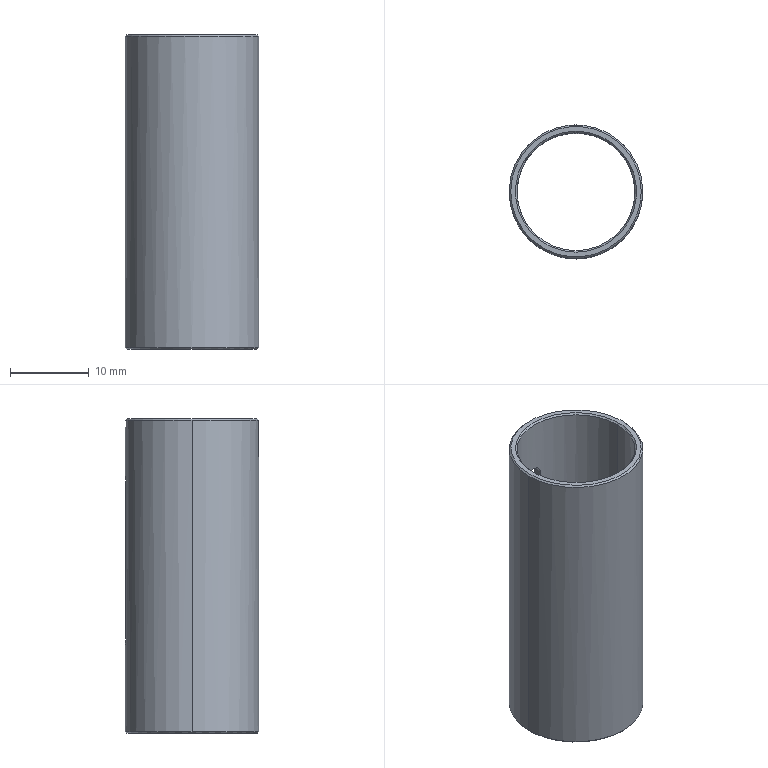Part | SolidWorks | features BaseBody 1, MoveFace 1 | 1 solid | 25 faces | box 17 x 17 x 40 mm | volume 1956 mm3 | cone 12 | cylinder 9 | plane 4 | commonest cylinder face diameters 15 x4 2 x3 17 x2
STEP:
#1=CARTESIAN_POINT('',(-1.,8.441,12.));
#2=VERTEX_POINT('',#1);
#3=CARTESIAN_POINT('',(0.,8.5,11.));
#4=VERTEX_POINT('',#3);
#5=CARTESIAN_POINT('',(-1.,8.441,12.));
#6=CARTESIAN_POINT('',(-1.,8.441,11.868));
#7=CARTESIAN_POINT('',(-0.9739,8.444,11.738));
#8=CARTESIAN_POINT('',(-0.8734,8.455,11.496));
#9=CARTESIAN_POINT('',(-0.7991,8.463,11.385));
#10=CARTESIAN_POINT('',(-0.6146,8.478,11.2));
#11=CARTESIAN_POINT('',(-0.5031,8.486,11.126));
#12=CARTESIAN_POINT('',(-0.2623,8.497,11.026));
#13=CARTESIAN_POINT('',(-0.1306,8.5,11.));
#14=CARTESIAN_POINT('',(0.,8.5,11.));
#15=B_SPLINE_CURVE_WITH_KNOTS('',3,(#5,#6,#7,#8,#9,#10,#11,#12,#13,#14),.UNSPECIFIED.,.F.,.F.,(4,2,2,2,4),(0.,0.0003912,0.0007825,0.001174,0.001565),.UNSPECIFIED.);
#16=EDGE_CURVE('',#2,#4,#15,.T.);
#17=ORIENTED_EDGE('',*,*,#16,.T.);
#18=CARTESIAN_POINT('',(1.,8.441,12.));
#19=VERTEX_POINT('',#18);
#20=CARTESIAN_POINT('',(0.,8.5,11.));
#21=CARTESIAN_POINT('',(0.1305,8.5,11.));
#22=CARTESIAN_POINT('',(0.2615,8.497,11.026));
#23=CARTESIAN_POINT('',(0.5036,8.486,11.126));
#24=CARTESIAN_POINT('',(0.6136,8.478,11.199));
#25=CARTESIAN_POINT('',(0.8002,8.463,11.386));
#26=CARTESIAN_POINT('',(0.8735,8.455,11.496));
#27=CARTESIAN_POINT('',(0.9739,8.444,11.738));
#28=CARTESIAN_POINT('',(1.,8.441,11.868));
#29=CARTESIAN_POINT('',(1.,8.441,12.));
#30=B_SPLINE_CURVE_WITH_KNOTS('',3,(#20,#21,#22,#23,#24,#25,#26,#27,#28,#29),.UNSPECIFIED.,.F.,.F.,(4,2,2,2,4),(0.001565,0.001956,0.002347,0.002738,0.003128),.UNSPECIFIED.);
#31=EDGE_CURVE('',#4,#19,#30,.T.);
#32=ORIENTED_EDGE('',*,*,#31,.T.);
#33=CARTESIAN_POINT('',(1.,8.441,32.));
#34=VERTEX_POINT('',#33);
#35=CARTESIAN_POINT('',(1.,8.441,40.));
#36=DIRECTION('',(0.,0.,1.));
#37=VECTOR('',#36,1000.);
#38=LINE('',#35,#37);
#39=EDGE_CURVE('',#19,#34,#38,.T.);
#40=ORIENTED_EDGE('',*,*,#39,.T.);
#41=CARTESIAN_POINT('',(-1.,8.441,32.));
#42=VERTEX_POINT('',#41);
#43=CARTESIAN_POINT('',(1.,8.441,32.));
#44=CARTESIAN_POINT('',(1.,8.441,32.132));
#45=CARTESIAN_POINT('',(0.9739,8.444,32.262));
#46=CARTESIAN_POINT('',(0.8735,8.455,32.504));
#47=CARTESIAN_POINT('',(0.7992,8.463,32.615));
#48=CARTESIAN_POINT('',(0.6149,8.478,32.799));
#49=CARTESIAN_POINT('',(0.5035,8.486,32.874));
#50=CARTESIAN_POINT('',(0.2629,8.497,32.974));
#51=CARTESIAN_POINT('',(0.1313,8.5,33.));
#52=CARTESIAN_POINT('',(-0.1298,8.5,33.));
#53=CARTESIAN_POINT('',(-0.2609,8.497,32.974));
#54=CARTESIAN_POINT('',(-0.5032,8.486,32.874));
#55=CARTESIAN_POINT('',(-0.6133,8.478,32.801));
#56=CARTESIAN_POINT('',(-0.8,8.463,32.614));
#57=CARTESIAN_POINT('',(-0.8734,8.455,32.504));
#58=CARTESIAN_POINT('',(-0.9738,8.444,32.262));
#59=CARTESIAN_POINT('',(-1.,8.441,32.132));
#60=CARTESIAN_POINT('',(-1.,8.441,32.));
#61=B_SPLINE_CURVE_WITH_KNOTS('',3,(#43,#44,#45,#46,#47,#48,#49,#50,#51,#52,#53,#54,#55,#56,#57,#58,#59,#60),.UNSPECIFIED.,.F.,.F.,(4,2,2,2,2,2,2,2,4),(0.,0.0003911,0.0007821,0.001173,0.001564,0.001955,0.002346,0.002737,0.003128),.UNSPECIFIED.);
#62=EDGE_CURVE('',#34,#42,#61,.T.);
#63=ORIENTED_EDGE('',*,*,#62,.T.);
#64=CARTESIAN_POINT('',(-1.,8.441,40.));
#65=DIRECTION('',(0.,0.,-1.));
#66=VECTOR('',#65,1000.);
#67=LINE('',#64,#66);
#68=EDGE_CURVE('',#42,#2,#67,.T.);
#69=ORIENTED_EDGE('',*,*,#68,.T.);
#70=EDGE_LOOP('',(#17,#32,#40,#63,#69));
#71=FACE_BOUND('',#70,.T.);
#72=CARTESIAN_POINT('',(-8.5,0.,39.8));
#73=VERTEX_POINT('',#72);
#74=CARTESIAN_POINT('',(8.5,0.,39.8));
#75=VERTEX_POINT('',#74);
#76=CARTESIAN_POINT('',(0.,0.,39.8));
#77=DIRECTION('',(0.,0.,-1.));
#78=DIRECTION('',(-1.,0.,0.));
#79=AXIS2_PLACEMENT_3D('',#76,#77,#78);
#80=CIRCLE('',#79,8.5);
#81=EDGE_CURVE('',#73,#75,#80,.T.);
#82=ORIENTED_EDGE('',*,*,#81,.T.);
#83=CARTESIAN_POINT('',(8.5,0.,0.2));
#84=VERTEX_POINT('',#83);
#85=CARTESIAN_POINT('',(8.5,0.,40.));
#86=DIRECTION('',(0.,0.,-1.));
#87=VECTOR('',#86,1000.);
#88=LINE('',#85,#87);
#89=EDGE_CURVE('',#75,#84,#88,.T.);
#90=ORIENTED_EDGE('',*,*,#89,.T.);
#91=CARTESIAN_POINT('',(0.,8.5,0.2));
#92=VERTEX_POINT('',#91);
#93=CARTESIAN_POINT('',(0.,0.,0.2));
#94=DIRECTION('',(0.,0.,1.));
#95=DIRECTION('',(-1.,0.,0.));
#96=AXIS2_PLACEMENT_3D('',#93,#94,#95);
#97=CIRCLE('',#96,8.5);
#98=EDGE_CURVE('',#84,#92,#97,.T.);
#99=ORIENTED_EDGE('',*,*,#98,.T.);
#100=CARTESIAN_POINT('',(-8.5,0.,0.2));
#101=VERTEX_POINT('',#100);
#102=CARTESIAN_POINT('',(0.,0.,0.2));
#103=DIRECTION('',(0.,0.,1.));
#104=DIRECTION('',(-1.,0.,0.));
#105=AXIS2_PLACEMENT_3D('',#102,#103,#104);
#106=CIRCLE('',#105,8.5);
#107=EDGE_CURVE('',#92,#101,#106,.T.);
#108=ORIENTED_EDGE('',*,*,#107,.T.);
#109=CARTESIAN_POINT('',(-8.5,0.,40.));
#110=DIRECTION('',(0.,0.,-1.));
#111=VECTOR('',#110,1000.);
#112=LINE('',#109,#111);
#113=EDGE_CURVE('',#73,#101,#112,.T.);
#114=ORIENTED_EDGE('',*,*,#113,.F.);
#115=EDGE_LOOP('',(#82,#90,#99,#108,#114));
#116=FACE_OUTER_BOUND('',#115,.T.);
#117=CARTESIAN_POINT('',(0.,0.,40.));
#118=DIRECTION('',(0.,0.,-1.));
#119=DIRECTION('',(-1.,0.,0.));
#120=AXIS2_PLACEMENT_3D('',#117,#118,#119);
#121=CYLINDRICAL_SURFACE('',#120,8.5);
#122=ADVANCED_FACE('',(#71,#116),#121,.T.);
#123=CARTESIAN_POINT('',(0.,-8.3,0.));
#124=VERTEX_POINT('',#123);
#125=CARTESIAN_POINT('',(0.,8.3,0.));
#126=VERTEX_POINT('',#125);
#127=CARTESIAN_POINT('',(0.,0.,0.));
#128=DIRECTION('',(0.,0.,1.));
#129=DIRECTION('',(0.,-1.,0.));
#130=AXIS2_PLACEMENT_3D('',#127,#128,#129);
#131=CIRCLE('',#130,8.3);
#132=EDGE_CURVE('',#124,#126,#131,.T.);
#133=ORIENTED_EDGE('',*,*,#132,.T.);
#134=CARTESIAN_POINT('',(0.,8.5,0.2));
#135=DIRECTION('',(0.,0.7071,0.7071));
#136=VECTOR('',#135,1000.);
#137=LINE('',#134,#136);
#138=EDGE_CURVE('',#126,#92,#137,.T.);
#139=ORIENTED_EDGE('',*,*,#138,.T.);
#140=ORIENTED_EDGE('',*,*,#98,.F.);
#141=CARTESIAN_POINT('',(0.,-8.5,0.2));
#142=VERTEX_POINT('',#141);
#143=CARTESIAN_POINT('',(0.,0.,0.2));
#144=DIRECTION('',(0.,0.,1.));
#145=DIRECTION('',(-1.,0.,0.));
#146=AXIS2_PLACEMENT_3D('',#143,#144,#145);
#147=CIRCLE('',#146,8.5);
#148=EDGE_CURVE('',#142,#84,#147,.T.);
#149=ORIENTED_EDGE('',*,*,#148,.F.);
#150=CARTESIAN_POINT('',(0.,-8.5,0.2));
#151=DIRECTION('',(0.,-0.7071,0.7071));
#152=VECTOR('',#151,1000.);
#153=LINE('',#150,#152);
#154=EDGE_CURVE('',#124,#142,#153,.T.);
#155=ORIENTED_EDGE('',*,*,#154,.F.);
#156=EDGE_LOOP('',(#133,#139,#140,#149,#155));
#157=FACE_OUTER_BOUND('',#156,.T.);
#158=CARTESIAN_POINT('',(0.,0.,0.2));
#159=DIRECTION('',(0.,0.,1.));
#160=DIRECTION('',(0.,-1.,0.));
#161=AXIS2_PLACEMENT_3D('',#158,#159,#160);
#162=CONICAL_SURFACE('',#161,8.5,0.7854);
#163=ADVANCED_FACE('',(#157),#162,.T.);
#164=CARTESIAN_POINT('',(-8.3,0.,40.));
#165=VERTEX_POINT('',#164);
#166=CARTESIAN_POINT('',(8.3,0.,40.));
#167=VERTEX_POINT('',#166);
#168=CARTESIAN_POINT('',(0.,0.,40.));
#169=DIRECTION('',(0.,0.,-1.));
#170=DIRECTION('',(-1.,0.,0.));
#171=AXIS2_PLACEMENT_3D('',#168,#169,#170);
#172=CIRCLE('',#171,8.3);
#173=EDGE_CURVE('',#165,#167,#172,.T.);
#174=ORIENTED_EDGE('',*,*,#173,.T.);
#175=CARTESIAN_POINT('',(8.5,0.,39.8));
#176=DIRECTION('',(0.7071,0.,-0.7071));
#177=VECTOR('',#176,1000.);
#178=LINE('',#175,#177);
#179=EDGE_CURVE('',#167,#75,#178,.T.);
#180=ORIENTED_EDGE('',*,*,#179,.T.);
#181=ORIENTED_EDGE('',*,*,#81,.F.);
#182=CARTESIAN_POINT('',(-8.5,0.,39.8));
#183=DIRECTION('',(-0.7071,0.,-0.7071));
#184=VECTOR('',#183,1000.);
#185=LINE('',#182,#184);
#186=EDGE_CURVE('',#165,#73,#185,.T.);
#187=ORIENTED_EDGE('',*,*,#186,.F.);
#188=EDGE_LOOP('',(#174,#180,#181,#187));
#189=FACE_OUTER_BOUND('',#188,.T.);
#190=CARTESIAN_POINT('',(0.,0.,39.8));
#191=DIRECTION('',(0.,0.,-1.));
#192=DIRECTION('',(-1.,0.,0.));
#193=AXIS2_PLACEMENT_3D('',#190,#191,#192);
#194=CONICAL_SURFACE('',#193,8.5,0.7854);
#195=ADVANCED_FACE('',(#189),#194,.T.);
#196=ORIENTED_EDGE('',*,*,#31,.F.);
#197=CARTESIAN_POINT('',(0.,7.5,11.));
#198=VERTEX_POINT('',#197);
#199=CARTESIAN_POINT('',(0.,8.5,11.));
#200=DIRECTION('',(0.,-1.,0.));
#201=VECTOR('',#200,1000.);
#202=LINE('',#199,#201);
#203=EDGE_CURVE('',#4,#198,#202,.T.);
#204=ORIENTED_EDGE('',*,*,#203,.T.);
#205=CARTESIAN_POINT('',(1.,7.433,12.));
#206=VERTEX_POINT('',#205);
#207=CARTESIAN_POINT('',(1.,7.433,12.));
#208=CARTESIAN_POINT('',(1.,7.433,11.868));
#209=CARTESIAN_POINT('',(0.9739,7.437,11.738));
#210=CARTESIAN_POINT('',(0.8734,7.449,11.496));
#211=CARTESIAN_POINT('',(0.799,7.458,11.385));
#212=CARTESIAN_POINT('',(0.6146,7.475,11.2));
#213=CARTESIAN_POINT('',(0.5031,7.484,11.126));
#214=CARTESIAN_POINT('',(0.2624,7.496,11.026));
#215=CARTESIAN_POINT('',(0.1306,7.5,11.));
#216=CARTESIAN_POINT('',(0.,7.5,11.));
#217=B_SPLINE_CURVE_WITH_KNOTS('',3,(#207,#208,#209,#210,#211,#212,#213,#214,#215,#216),.UNSPECIFIED.,.F.,.F.,(4,2,2,2,4),(0.,0.0003913,0.0007827,0.001174,0.001565),.UNSPECIFIED.);
#218=EDGE_CURVE('',#206,#198,#217,.T.);
#219=ORIENTED_EDGE('',*,*,#218,.F.);
#220=CARTESIAN_POINT('',(1.,8.5,12.));
#221=DIRECTION('',(0.,-1.,0.));
#222=VECTOR('',#221,1000.);
#223=LINE('',#220,#222);
#224=EDGE_CURVE('',#19,#206,#223,.T.);
#225=ORIENTED_EDGE('',*,*,#224,.F.);
#226=EDGE_LOOP('',(#196,#204,#219,#225));
#227=FACE_OUTER_BOUND('',#226,.T.);
#228=CARTESIAN_POINT('',(0.,8.5,12.));
#229=DIRECTION('',(0.,-1.,0.));
#230=DIRECTION('',(0.,0.,-1.));
#231=AXIS2_PLACEMENT_3D('',#228,#229,#230);
#232=CYLINDRICAL_SURFACE('',#231,1.);
#233=ADVANCED_FACE('',(#227),#232,.F.);
#234=CARTESIAN_POINT('',(7.5,0.,0.2));
#235=VERTEX_POINT('',#234);
#236=CARTESIAN_POINT('',(-7.5,0.,0.2));
#237=VERTEX_POINT('',#236);
#238=CARTESIAN_POINT('',(0.,0.,0.2));
#239=DIRECTION('',(0.,0.,-1.));
#240=DIRECTION('',(-1.,0.,0.));
#241=AXIS2_PLACEMENT_3D('',#238,#239,#240);
#242=CIRCLE('',#241,7.5);
#243=EDGE_CURVE('',#235,#237,#242,.T.);
#244=ORIENTED_EDGE('',*,*,#243,.F.);
#245=CARTESIAN_POINT('',(7.7,0.,0.));
#246=VERTEX_POINT('',#245);
#247=CARTESIAN_POINT('',(7.7,0.,0.));
#248=DIRECTION('',(0.7071,0.,-0.7071));
#249=VECTOR('',#248,1000.);
#250=LINE('',#247,#249);
#251=EDGE_CURVE('',#235,#246,#250,.T.);
#252=ORIENTED_EDGE('',*,*,#251,.T.);
#253=CARTESIAN_POINT('',(-7.7,0.,0.));
#254=VERTEX_POINT('',#253);
#255=CARTESIAN_POINT('',(0.,0.,0.));
#256=DIRECTION('',(0.,0.,-1.));
#257=DIRECTION('',(-1.,0.,0.));
#258=AXIS2_PLACEMENT_3D('',#255,#256,#257);
#259=CIRCLE('',#258,7.7);
#260=EDGE_CURVE('',#246,#254,#259,.T.);
#261=ORIENTED_EDGE('',*,*,#260,.T.);
#262=CARTESIAN_POINT('',(-7.7,0.,0.));
#263=DIRECTION('',(-0.7071,0.,-0.7071));
#264=VECTOR('',#263,1000.);
#265=LINE('',#262,#264);
#266=EDGE_CURVE('',#237,#254,#265,.T.);
#267=ORIENTED_EDGE('',*,*,#266,.F.);
#268=EDGE_LOOP('',(#244,#252,#261,#267));
#269=FACE_OUTER_BOUND('',#268,.T.);
#270=CARTESIAN_POINT('',(0.,0.,0.));
#271=DIRECTION('',(0.,0.,-1.));
#272=DIRECTION('',(-1.,0.,0.));
#273=AXIS2_PLACEMENT_3D('',#270,#271,#272);
#274=CONICAL_SURFACE('',#273,7.7,0.7854);
#275=ADVANCED_FACE('',(#269),#274,.F.);
#276=CARTESIAN_POINT('',(7.5,0.,39.8));
#277=VERTEX_POINT('',#276);
#278=CARTESIAN_POINT('',(0.,-7.5,39.8));
#279=VERTEX_POINT('',#278);
#280=CARTESIAN_POINT('',(0.,0.,39.8));
#281=DIRECTION('',(0.,0.,-1.));
#282=DIRECTION('',(-1.,0.,0.));
#283=AXIS2_PLACEMENT_3D('',#280,#281,#282);
#284=CIRCLE('',#283,7.5);
#285=EDGE_CURVE('',#277,#279,#284,.T.);
#286=ORIENTED_EDGE('',*,*,#285,.F.);
#287=CARTESIAN_POINT('',(7.5,0.,2.289));
#288=VERTEX_POINT('',#287);
#289=CARTESIAN_POINT('',(7.5,0.,40.));
#290=DIRECTION('',(0.,0.,-1.));
#291=VECTOR('',#290,1000.);
#292=LINE('',#289,#291);
#293=EDGE_CURVE('',#277,#288,#292,.T.);
#294=ORIENTED_EDGE('',*,*,#293,.T.);
#295=CARTESIAN_POINT('',(-7.5,0.,2.289));
#296=VERTEX_POINT('',#295);
#297=CARTESIAN_POINT('',(0.,0.,2.289));
#298=DIRECTION('',(0.,0.,1.));
#299=DIRECTION('',(-1.,0.,0.));
#300=AXIS2_PLACEMENT_3D('',#297,#298,#299);
#301=CIRCLE('',#300,7.5);
#302=EDGE_CURVE('',#296,#288,#301,.T.);
#303=ORIENTED_EDGE('',*,*,#302,.F.);
#304=CARTESIAN_POINT('',(-7.5,0.,39.8));
#305=VERTEX_POINT('',#304);
#306=CARTESIAN_POINT('',(-7.5,0.,40.));
#307=DIRECTION('',(0.,0.,-1.));
#308=VECTOR('',#307,1000.);
#309=LINE('',#306,#308);
#310=EDGE_CURVE('',#305,#296,#309,.T.);
#311=ORIENTED_EDGE('',*,*,#310,.F.);
#312=CARTESIAN_POINT('',(0.,0.,39.8));
#313=DIRECTION('',(0.,0.,-1.));
#314=DIRECTION('',(-1.,0.,0.));
#315=AXIS2_PLACEMENT_3D('',#312,#313,#314);
#316=CIRCLE('',#315,7.5);
#317=EDGE_CURVE('',#279,#305,#316,.T.);
#318=ORIENTED_EDGE('',*,*,#317,.F.);
#319=EDGE_LOOP('',(#286,#294,#303,#311,#318));
#320=FACE_OUTER_BOUND('',#319,.T.);
#321=CARTESIAN_POINT('',(0.,0.,40.));
#322=DIRECTION('',(0.,0.,-1.));
#323=DIRECTION('',(-1.,0.,0.));
#324=AXIS2_PLACEMENT_3D('',#321,#322,#323);
#325=CYLINDRICAL_SURFACE('',#324,7.5);
#326=ADVANCED_FACE('',(#320),#325,.F.);
#327=ORIENTED_EDGE('',*,*,#317,.T.);
#328=CARTESIAN_POINT('',(0.,7.5,39.8));
#329=VERTEX_POINT('',#328);
#330=CARTESIAN_POINT('',(0.,0.,39.8));
#331=DIRECTION('',(0.,0.,-1.));
#332=DIRECTION('',(-1.,0.,0.));
#333=AXIS2_PLACEMENT_3D('',#330,#331,#332);
#334=CIRCLE('',#333,7.5);
#335=EDGE_CURVE('',#305,#329,#334,.T.);
#336=ORIENTED_EDGE('',*,*,#335,.T.);
#337=CARTESIAN_POINT('',(0.,7.7,40.));
#338=VERTEX_POINT('',#337);
#339=CARTESIAN_POINT('',(0.,7.7,40.));
#340=DIRECTION('',(0.,0.7071,0.7071));
#341=VECTOR('',#340,1000.);
#342=LINE('',#339,#341);
#343=EDGE_CURVE('',#329,#338,#342,.T.);
#344=ORIENTED_EDGE('',*,*,#343,.T.);
#345=CARTESIAN_POINT('',(0.,-7.7,40.));
#346=VERTEX_POINT('',#345);
#347=CARTESIAN_POINT('',(0.,0.,40.));
#348=DIRECTION('',(0.,0.,-1.));
#349=DIRECTION('',(0.,-1.,0.));
#350=AXIS2_PLACEMENT_3D('',#347,#348,#349);
#351=CIRCLE('',#350,7.7);
#352=EDGE_CURVE('',#346,#338,#351,.T.);
#353=ORIENTED_EDGE('',*,*,#352,.F.);
#354=CARTESIAN_POINT('',(0.,-7.7,40.));
#355=DIRECTION('',(0.,-0.7071,0.7071));
#356=VECTOR('',#355,1000.);
#357=LINE('',#354,#356);
#358=EDGE_CURVE('',#279,#346,#357,.T.);
#359=ORIENTED_EDGE('',*,*,#358,.F.);
#360=EDGE_LOOP('',(#327,#336,#344,#353,#359));
#361=FACE_OUTER_BOUND('',#360,.T.);
#362=CARTESIAN_POINT('',(0.,0.,40.));
#363=DIRECTION('',(0.,0.,1.));
#364=DIRECTION('',(0.,-1.,0.));
#365=AXIS2_PLACEMENT_3D('',#362,#363,#364);
#366=CONICAL_SURFACE('',#365,7.7,0.7854);
#367=ADVANCED_FACE('',(#361),#366,.F.);
#368=CARTESIAN_POINT('',(7.5,0.,1.711));
#369=VERTEX_POINT('',#368);
#370=CARTESIAN_POINT('',(-7.5,0.,1.711));
#371=VERTEX_POINT('',#370);
#372=CARTESIAN_POINT('',(0.,0.,1.711));
#373=DIRECTION('',(0.,0.,-1.));
#374=DIRECTION('',(-1.,0.,0.));
#375=AXIS2_PLACEMENT_3D('',#372,#373,#374);
#376=CIRCLE('',#375,7.5);
#377=EDGE_CURVE('',#369,#371,#376,.T.);
#378=ORIENTED_EDGE('',*,*,#377,.F.);
#379=CARTESIAN_POINT('',(7.5,0.,40.));
#380=DIRECTION('',(0.,0.,-1.));
#381=VECTOR('',#380,1000.);
#382=LINE('',#379,#381);
#383=EDGE_CURVE('',#369,#235,#382,.T.);
#384=ORIENTED_EDGE('',*,*,#383,.T.);
#385=ORIENTED_EDGE('',*,*,#243,.T.);
#386=CARTESIAN_POINT('',(-7.5,0.,40.));
#387=DIRECTION('',(0.,0.,-1.));
#388=VECTOR('',#387,1000.);
#389=LINE('',#386,#388);
#390=EDGE_CURVE('',#371,#237,#389,.T.);
#391=ORIENTED_EDGE('',*,*,#390,.F.);
#392=EDGE_LOOP('',(#378,#384,#385,#391));
#393=FACE_OUTER_BOUND('',#392,.T.);
#394=CARTESIAN_POINT('',(0.,0.,40.));
#395=DIRECTION('',(0.,0.,-1.));
#396=DIRECTION('',(-1.,0.,0.));
#397=AXIS2_PLACEMENT_3D('',#394,#395,#396);
#398=CYLINDRICAL_SURFACE('',#397,7.5);
#399=ADVANCED_FACE('',(#393),#398,.F.);
#400=ORIENTED_EDGE('',*,*,#302,.T.);
#401=CARTESIAN_POINT('',(8.,0.,2.));
#402=VERTEX_POINT('',#401);
#403=CARTESIAN_POINT('',(8.,0.,2.));
#404=DIRECTION('',(0.866,0.,-0.5));
#405=VECTOR('',#404,1000.);
#406=LINE('',#403,#405);
#407=EDGE_CURVE('',#288,#402,#406,.T.);
#408=ORIENTED_EDGE('',*,*,#407,.T.);
#409=CARTESIAN_POINT('',(-8.,0.,2.));
#410=VERTEX_POINT('',#409);
#411=CARTESIAN_POINT('',(0.,0.,2.));
#412=DIRECTION('',(0.,0.,1.));
#413=DIRECTION('',(-1.,0.,0.));
#414=AXIS2_PLACEMENT_3D('',#411,#412,#413);
#415=CIRCLE('',#414,8.);
#416=EDGE_CURVE('',#410,#402,#415,.T.);
#417=ORIENTED_EDGE('',*,*,#416,.F.);
#418=CARTESIAN_POINT('',(-8.,0.,2.));
#419=DIRECTION('',(-0.866,0.,-0.5));
#420=VECTOR('',#419,1000.);
#421=LINE('',#418,#420);
#422=EDGE_CURVE('',#296,#410,#421,.T.);
#423=ORIENTED_EDGE('',*,*,#422,.F.);
#424=EDGE_LOOP('',(#400,#408,#417,#423));
#425=FACE_OUTER_BOUND('',#424,.T.);
#426=CARTESIAN_POINT('',(0.,0.,2.));
#427=DIRECTION('',(0.,0.,-1.));
#428=DIRECTION('',(-1.,0.,0.));
#429=AXIS2_PLACEMENT_3D('',#426,#427,#428);
#430=CONICAL_SURFACE('',#429,8.,1.047);
#431=ADVANCED_FACE('',(#425),#430,.F.);
#432=ORIENTED_EDGE('',*,*,#377,.T.);
#433=CARTESIAN_POINT('',(-8.,0.,2.));
#434=DIRECTION('',(-0.866,0.,0.5));
#435=VECTOR('',#434,1000.);
#436=LINE('',#433,#435);
#437=EDGE_CURVE('',#371,#410,#436,.T.);
#438=ORIENTED_EDGE('',*,*,#437,.T.);
#439=ORIENTED_EDGE('',*,*,#416,.T.);
#440=CARTESIAN_POINT('',(8.,0.,2.));
#441=DIRECTION('',(0.866,0.,0.5));
#442=VECTOR('',#441,1000.);
#443=LINE('',#440,#442);
#444=EDGE_CURVE('',#369,#402,#443,.T.);
#445=ORIENTED_EDGE('',*,*,#444,.F.);
#446=EDGE_LOOP('',(#432,#438,#439,#445));
#447=FACE_OUTER_BOUND('',#446,.T.);
#448=CARTESIAN_POINT('',(0.,0.,2.));
#449=DIRECTION('',(0.,0.,1.));
#450=DIRECTION('',(1.,0.,0.));
#451=AXIS2_PLACEMENT_3D('',#448,#449,#450);
#452=CONICAL_SURFACE('',#451,8.,1.047);
#453=ADVANCED_FACE('',(#447),#452,.F.);
#454=ORIENTED_EDGE('',*,*,#89,.F.);
#455=CARTESIAN_POINT('',(0.,0.,39.8));
#456=DIRECTION('',(0.,0.,-1.));
#457=DIRECTION('',(-1.,0.,0.));
#458=AXIS2_PLACEMENT_3D('',#455,#456,#457);
#459=CIRCLE('',#458,8.5);
#460=EDGE_CURVE('',#75,#73,#459,.T.);
#461=ORIENTED_EDGE('',*,*,#460,.T.);
#462=ORIENTED_EDGE('',*,*,#113,.T.);
#463=CARTESIAN_POINT('',(0.,0.,0.2));
#464=DIRECTION('',(0.,0.,1.));
#465=DIRECTION('',(-1.,0.,0.));
#466=AXIS2_PLACEMENT_3D('',#463,#464,#465);
#467=CIRCLE('',#466,8.5);
#468=EDGE_CURVE('',#101,#142,#467,.T.);
#469=ORIENTED_EDGE('',*,*,#468,.T.);
#470=ORIENTED_EDGE('',*,*,#148,.T.);
#471=EDGE_LOOP('',(#454,#461,#462,#469,#470));
#472=FACE_OUTER_BOUND('',#471,.T.);
#473=CARTESIAN_POINT('',(0.,0.,40.));
#474=DIRECTION('',(0.,0.,-1.));
#475=DIRECTION('',(-1.,0.,0.));
#476=AXIS2_PLACEMENT_3D('',#473,#474,#475);
#477=CYLINDRICAL_SURFACE('',#476,8.5);
#478=ADVANCED_FACE('',(#472),#477,.T.);
#479=ORIENTED_EDGE('',*,*,#138,.F.);
#480=CARTESIAN_POINT('',(0.,0.,0.));
#481=DIRECTION('',(0.,0.,1.));
#482=DIRECTION('',(0.,-1.,0.));
#483=AXIS2_PLACEMENT_3D('',#480,#481,#482);
#484=CIRCLE('',#483,8.3);
#485=EDGE_CURVE('',#126,#124,#484,.T.);
#486=ORIENTED_EDGE('',*,*,#485,.T.);
#487=ORIENTED_EDGE('',*,*,#154,.T.);
#488=ORIENTED_EDGE('',*,*,#468,.F.);
#489=ORIENTED_EDGE('',*,*,#107,.F.);
#490=EDGE_LOOP('',(#479,#486,#487,#488,#489));
#491=FACE_OUTER_BOUND('',#490,.T.);
#492=CARTESIAN_POINT('',(0.,0.,0.2));
#493=DIRECTION('',(0.,0.,1.));
#494=DIRECTION('',(0.,-1.,0.));
#495=AXIS2_PLACEMENT_3D('',#492,#493,#494);
#496=CONICAL_SURFACE('',#495,8.5,0.7854);
#497=ADVANCED_FACE('',(#491),#496,.T.);
#498=ORIENTED_EDGE('',*,*,#179,.F.);
#499=CARTESIAN_POINT('',(0.,0.,40.));
#500=DIRECTION('',(0.,0.,-1.));
#501=DIRECTION('',(-1.,0.,0.));
#502=AXIS2_PLACEMENT_3D('',#499,#500,#501);
#503=CIRCLE('',#502,8.3);
#504=EDGE_CURVE('',#167,#165,#503,.T.);
#505=ORIENTED_EDGE('',*,*,#504,.T.);
#506=ORIENTED_EDGE('',*,*,#186,.T.);
#507=ORIENTED_EDGE('',*,*,#460,.F.);
#508=EDGE_LOOP('',(#498,#505,#506,#507));
#509=FACE_OUTER_BOUND('',#508,.T.);
#510=CARTESIAN_POINT('',(0.,0.,39.8));
#511=DIRECTION('',(0.,0.,-1.));
#512=DIRECTION('',(-1.,0.,0.));
#513=AXIS2_PLACEMENT_3D('',#510,#511,#512);
#514=CONICAL_SURFACE('',#513,8.5,0.7854);
#515=ADVANCED_FACE('',(#509),#514,.T.);
#516=ORIENTED_EDGE('',*,*,#132,.F.);
#517=ORIENTED_EDGE('',*,*,#485,.F.);
#518=EDGE_LOOP('',(#516,#517));
#519=FACE_OUTER_BOUND('',#518,.T.);
#520=CARTESIAN_POINT('',(0.,0.,0.));
#521=DIRECTION('',(0.,0.,-1.));
#522=DIRECTION('',(-1.,0.,0.));
#523=AXIS2_PLACEMENT_3D('',#520,#521,#522);
#524=CIRCLE('',#523,7.7);
#525=EDGE_CURVE('',#254,#246,#524,.T.);
#526=ORIENTED_EDGE('',*,*,#525,.F.);
#527=ORIENTED_EDGE('',*,*,#260,.F.);
#528=EDGE_LOOP('',(#526,#527));
#529=FACE_BOUND('',#528,.T.);
#530=CARTESIAN_POINT('',(0.,0.,0.));
#531=DIRECTION('',(0.,0.,1.));
#532=DIRECTION('',(1.,0.,0.));
#533=AXIS2_PLACEMENT_3D('',#530,#531,#532);
#534=PLANE('',#533);
#535=ADVANCED_FACE('',(#519,#529),#534,.F.);
#536=CARTESIAN_POINT('',(1.,7.433,32.));
#537=VERTEX_POINT('',#536);
#538=CARTESIAN_POINT('',(1.,7.433,18.));
#539=DIRECTION('',(0.,0.,1.));
#540=VECTOR('',#539,1000.);
#541=LINE('',#538,#540);
#542=EDGE_CURVE('',#206,#537,#541,.T.);
#543=ORIENTED_EDGE('',*,*,#542,.T.);
#544=CARTESIAN_POINT('',(1.,8.5,32.));
#545=DIRECTION('',(0.,1.,0.));
#546=VECTOR('',#545,1000.);
#547=LINE('',#544,#546);
#548=EDGE_CURVE('',#537,#34,#547,.T.);
#549=ORIENTED_EDGE('',*,*,#548,.T.);
#550=ORIENTED_EDGE('',*,*,#39,.F.);
#551=ORIENTED_EDGE('',*,*,#224,.T.);
#552=EDGE_LOOP('',(#543,#549,#550,#551));
#553=FACE_OUTER_BOUND('',#552,.T.);
#554=CARTESIAN_POINT('',(1.,8.5,18.));
#555=DIRECTION('',(-1.,0.,0.));
#556=DIRECTION('',(0.,0.,1.));
#557=AXIS2_PLACEMENT_3D('',#554,#555,#556);
#558=PLANE('',#557);
#559=ADVANCED_FACE('',(#553),#558,.T.);
#560=ORIENTED_EDGE('',*,*,#203,.F.);
#561=ORIENTED_EDGE('',*,*,#16,.F.);
#562=CARTESIAN_POINT('',(-1.,7.433,12.));
#563=VERTEX_POINT('',#562);
#564=CARTESIAN_POINT('',(-1.,8.5,12.));
#565=DIRECTION('',(0.,1.,0.));
#566=VECTOR('',#565,1000.);
#567=LINE('',#564,#566);
#568=EDGE_CURVE('',#563,#2,#567,.T.);
#569=ORIENTED_EDGE('',*,*,#568,.F.);
#570=CARTESIAN_POINT('',(0.,7.5,11.));
#571=CARTESIAN_POINT('',(-0.1305,7.5,11.));
#572=CARTESIAN_POINT('',(-0.2616,7.496,11.026));
#573=CARTESIAN_POINT('',(-0.5037,7.484,11.126));
#574=CARTESIAN_POINT('',(-0.6137,7.475,11.2));
#575=CARTESIAN_POINT('',(-0.8001,7.458,11.386));
#576=CARTESIAN_POINT('',(-0.8735,7.449,11.496));
#577=CARTESIAN_POINT('',(-0.9738,7.437,11.738));
#578=CARTESIAN_POINT('',(-1.,7.433,11.868));
#579=CARTESIAN_POINT('',(-1.,7.433,12.));
#580=B_SPLINE_CURVE_WITH_KNOTS('',3,(#570,#571,#572,#573,#574,#575,#576,#577,#578,#579),.UNSPECIFIED.,.F.,.F.,(4,2,2,2,4),(0.001565,0.001956,0.002347,0.002738,0.003129),.UNSPECIFIED.);
#581=EDGE_CURVE('',#198,#563,#580,.T.);
#582=ORIENTED_EDGE('',*,*,#581,.F.);
#583=EDGE_LOOP('',(#560,#561,#569,#582));
#584=FACE_OUTER_BOUND('',#583,.T.);
#585=CARTESIAN_POINT('',(0.,8.5,12.));
#586=DIRECTION('',(0.,-1.,0.));
#587=DIRECTION('',(0.,0.,-1.));
#588=AXIS2_PLACEMENT_3D('',#585,#586,#587);
#589=CYLINDRICAL_SURFACE('',#588,1.);
#590=ADVANCED_FACE('',(#584),#589,.F.);
#591=CARTESIAN_POINT('',(-1.,7.433,32.));
#592=VERTEX_POINT('',#591);
#593=CARTESIAN_POINT('',(-1.,7.433,18.));
#594=DIRECTION('',(0.,0.,-1.));
#595=VECTOR('',#594,1000.);
#596=LINE('',#593,#595);
#597=EDGE_CURVE('',#592,#563,#596,.T.);
#598=ORIENTED_EDGE('',*,*,#597,.T.);
#599=ORIENTED_EDGE('',*,*,#568,.T.);
#600=ORIENTED_EDGE('',*,*,#68,.F.);
#601=CARTESIAN_POINT('',(-1.,8.5,32.));
#602=DIRECTION('',(0.,-1.,0.));
#603=VECTOR('',#602,1000.);
#604=LINE('',#601,#603);
#605=EDGE_CURVE('',#42,#592,#604,.T.);
#606=ORIENTED_EDGE('',*,*,#605,.T.);
#607=EDGE_LOOP('',(#598,#599,#600,#606));
#608=FACE_OUTER_BOUND('',#607,.T.);
#609=CARTESIAN_POINT('',(-1.,8.5,18.));
#610=DIRECTION('',(1.,0.,0.));
#611=DIRECTION('',(0.,0.,-1.));
#612=AXIS2_PLACEMENT_3D('',#609,#610,#611);
#613=PLANE('',#612);
#614=ADVANCED_FACE('',(#608),#613,.T.);
#615=ORIENTED_EDGE('',*,*,#548,.F.);
#616=CARTESIAN_POINT('',(-1.,7.433,32.));
#617=CARTESIAN_POINT('',(-1.,7.433,32.132));
#618=CARTESIAN_POINT('',(-0.9739,7.437,32.262));
#619=CARTESIAN_POINT('',(-0.8735,7.449,32.504));
#620=CARTESIAN_POINT('',(-0.7992,7.458,32.615));
#621=CARTESIAN_POINT('',(-0.615,7.475,32.799));
#622=CARTESIAN_POINT('',(-0.5035,7.484,32.874));
#623=CARTESIAN_POINT('',(-0.263,7.496,32.974));
#624=CARTESIAN_POINT('',(-0.1313,7.5,33.));
#625=CARTESIAN_POINT('',(0.1298,7.5,33.));
#626=CARTESIAN_POINT('',(0.261,7.496,32.974));
#627=CARTESIAN_POINT('',(0.5033,7.484,32.874));
#628=CARTESIAN_POINT('',(0.6133,7.475,32.801));
#629=CARTESIAN_POINT('',(0.8,7.458,32.614));
#630=CARTESIAN_POINT('',(0.8733,7.449,32.504));
#631=CARTESIAN_POINT('',(0.9738,7.437,32.262));
#632=CARTESIAN_POINT('',(1.,7.433,32.132));
#633=CARTESIAN_POINT('',(1.,7.433,32.));
#634=B_SPLINE_CURVE_WITH_KNOTS('',3,(#616,#617,#618,#619,#620,#621,#622,#623,#624,#625,#626,#627,#628,#629,#630,#631,#632,#633),.UNSPECIFIED.,.F.,.F.,(4,2,2,2,2,2,2,2,4),(0.,0.0003912,0.0007823,0.001173,0.001565,0.001956,0.002347,0.002738,0.003129),.UNSPECIFIED.);
#635=EDGE_CURVE('',#592,#537,#634,.T.);
#636=ORIENTED_EDGE('',*,*,#635,.F.);
#637=ORIENTED_EDGE('',*,*,#605,.F.);
#638=ORIENTED_EDGE('',*,*,#62,.F.);
#639=EDGE_LOOP('',(#615,#636,#637,#638));
#640=FACE_OUTER_BOUND('',#639,.T.);
#641=CARTESIAN_POINT('',(0.,8.5,32.));
#642=DIRECTION('',(0.,-1.,0.));
#643=DIRECTION('',(0.,0.,-1.));
#644=AXIS2_PLACEMENT_3D('',#641,#642,#643);
#645=CYLINDRICAL_SURFACE('',#644,1.);
#646=ADVANCED_FACE('',(#640),#645,.F.);
#647=ORIENTED_EDGE('',*,*,#173,.F.);
#648=ORIENTED_EDGE('',*,*,#504,.F.);
#649=EDGE_LOOP('',(#647,#648));
#650=FACE_OUTER_BOUND('',#649,.T.);
#651=ORIENTED_EDGE('',*,*,#352,.T.);
#652=CARTESIAN_POINT('',(0.,0.,40.));
#653=DIRECTION('',(0.,0.,-1.));
#654=DIRECTION('',(0.,-1.,0.));
#655=AXIS2_PLACEMENT_3D('',#652,#653,#654);
#656=CIRCLE('',#655,7.7);
#657=EDGE_CURVE('',#338,#346,#656,.T.);
#658=ORIENTED_EDGE('',*,*,#657,.T.);
#659=EDGE_LOOP('',(#651,#658));
#660=FACE_BOUND('',#659,.T.);
#661=CARTESIAN_POINT('',(0.,0.,40.));
#662=DIRECTION('',(0.,0.,1.));
#663=DIRECTION('',(1.,0.,0.));
#664=AXIS2_PLACEMENT_3D('',#661,#662,#663);
#665=PLANE('',#664);
#666=ADVANCED_FACE('',(#650,#660),#665,.T.);
#667=ORIENTED_EDGE('',*,*,#251,.F.);
#668=CARTESIAN_POINT('',(0.,0.,0.2));
#669=DIRECTION('',(0.,0.,-1.));
#670=DIRECTION('',(-1.,0.,0.));
#671=AXIS2_PLACEMENT_3D('',#668,#669,#670);
#672=CIRCLE('',#671,7.5);
#673=EDGE_CURVE('',#237,#235,#672,.T.);
#674=ORIENTED_EDGE('',*,*,#673,.F.);
#675=ORIENTED_EDGE('',*,*,#266,.T.);
#676=ORIENTED_EDGE('',*,*,#525,.T.);
#677=EDGE_LOOP('',(#667,#674,#675,#676));
#678=FACE_OUTER_BOUND('',#677,.T.);
#679=CARTESIAN_POINT('',(0.,0.,0.));
#680=DIRECTION('',(0.,0.,-1.));
#681=DIRECTION('',(-1.,0.,0.));
#682=AXIS2_PLACEMENT_3D('',#679,#680,#681);
#683=CONICAL_SURFACE('',#682,7.7,0.7854);
#684=ADVANCED_FACE('',(#678),#683,.F.);
#685=ORIENTED_EDGE('',*,*,#293,.F.);
#686=CARTESIAN_POINT('',(0.,0.,39.8));
#687=DIRECTION('',(0.,0.,-1.));
#688=DIRECTION('',(-1.,0.,0.));
#689=AXIS2_PLACEMENT_3D('',#686,#687,#688);
#690=CIRCLE('',#689,7.5);
#691=EDGE_CURVE('',#329,#277,#690,.T.);
#692=ORIENTED_EDGE('',*,*,#691,.F.);
#693=ORIENTED_EDGE('',*,*,#335,.F.);
#694=ORIENTED_EDGE('',*,*,#310,.T.);
#695=CARTESIAN_POINT('',(0.,0.,2.289));
#696=DIRECTION('',(0.,0.,1.));
#697=DIRECTION('',(-1.,0.,0.));
#698=AXIS2_PLACEMENT_3D('',#695,#696,#697);
#699=CIRCLE('',#698,7.5);
#700=EDGE_CURVE('',#288,#296,#699,.T.);
#701=ORIENTED_EDGE('',*,*,#700,.F.);
#702=EDGE_LOOP('',(#685,#692,#693,#694,#701));
#703=FACE_OUTER_BOUND('',#702,.T.);
#704=ORIENTED_EDGE('',*,*,#218,.T.);
#705=ORIENTED_EDGE('',*,*,#581,.T.);
#706=ORIENTED_EDGE('',*,*,#597,.F.);
#707=ORIENTED_EDGE('',*,*,#635,.T.);
#708=ORIENTED_EDGE('',*,*,#542,.F.);
#709=EDGE_LOOP('',(#704,#705,#706,#707,#708));
#710=FACE_BOUND('',#709,.T.);
#711=CARTESIAN_POINT('',(0.,0.,40.));
#712=DIRECTION('',(0.,0.,-1.));
#713=DIRECTION('',(-1.,0.,0.));
#714=AXIS2_PLACEMENT_3D('',#711,#712,#713);
#715=CYLINDRICAL_SURFACE('',#714,7.5);
#716=ADVANCED_FACE('',(#703,#710),#715,.F.);
#717=ORIENTED_EDGE('',*,*,#343,.F.);
#718=ORIENTED_EDGE('',*,*,#691,.T.);
#719=ORIENTED_EDGE('',*,*,#285,.T.);
#720=ORIENTED_EDGE('',*,*,#358,.T.);
#721=ORIENTED_EDGE('',*,*,#657,.F.);
#722=EDGE_LOOP('',(#717,#718,#719,#720,#721));
#723=FACE_OUTER_BOUND('',#722,.T.);
#724=CARTESIAN_POINT('',(0.,0.,40.));
#725=DIRECTION('',(0.,0.,1.));
#726=DIRECTION('',(0.,-1.,0.));
#727=AXIS2_PLACEMENT_3D('',#724,#725,#726);
#728=CONICAL_SURFACE('',#727,7.7,0.7854);
#729=ADVANCED_FACE('',(#723),#728,.F.);
#730=ORIENTED_EDGE('',*,*,#383,.F.);
#731=CARTESIAN_POINT('',(0.,0.,1.711));
#732=DIRECTION('',(0.,0.,-1.));
#733=DIRECTION('',(-1.,0.,0.));
#734=AXIS2_PLACEMENT_3D('',#731,#732,#733);
#735=CIRCLE('',#734,7.5);
#736=EDGE_CURVE('',#371,#369,#735,.T.);
#737=ORIENTED_EDGE('',*,*,#736,.F.);
#738=ORIENTED_EDGE('',*,*,#390,.T.);
#739=ORIENTED_EDGE('',*,*,#673,.T.);
#740=EDGE_LOOP('',(#730,#737,#738,#739));
#741=FACE_OUTER_BOUND('',#740,.T.);
#742=CARTESIAN_POINT('',(0.,0.,40.));
#743=DIRECTION('',(0.,0.,-1.));
#744=DIRECTION('',(-1.,0.,0.));
#745=AXIS2_PLACEMENT_3D('',#742,#743,#744);
#746=CYLINDRICAL_SURFACE('',#745,7.5);
#747=ADVANCED_FACE('',(#741),#746,.F.);
#748=ORIENTED_EDGE('',*,*,#407,.F.);
#749=ORIENTED_EDGE('',*,*,#700,.T.);
#750=ORIENTED_EDGE('',*,*,#422,.T.);
#751=CARTESIAN_POINT('',(0.,0.,2.));
#752=DIRECTION('',(0.,0.,1.));
#753=DIRECTION('',(-1.,0.,0.));
#754=AXIS2_PLACEMENT_3D('',#751,#752,#753);
#755=CIRCLE('',#754,8.);
#756=EDGE_CURVE('',#402,#410,#755,.T.);
#757=ORIENTED_EDGE('',*,*,#756,.F.);
#758=EDGE_LOOP('',(#748,#749,#750,#757));
#759=FACE_OUTER_BOUND('',#758,.T.);
#760=CARTESIAN_POINT('',(0.,0.,2.));
#761=DIRECTION('',(0.,0.,-1.));
#762=DIRECTION('',(-1.,0.,0.));
#763=AXIS2_PLACEMENT_3D('',#760,#761,#762);
#764=CONICAL_SURFACE('',#763,8.,1.047);
#765=ADVANCED_FACE('',(#759),#764,.F.);
#766=ORIENTED_EDGE('',*,*,#437,.F.);
#767=ORIENTED_EDGE('',*,*,#736,.T.);
#768=ORIENTED_EDGE('',*,*,#444,.T.);
#769=ORIENTED_EDGE('',*,*,#756,.T.);
#770=EDGE_LOOP('',(#766,#767,#768,#769));
#771=FACE_OUTER_BOUND('',#770,.T.);
#772=CARTESIAN_POINT('',(0.,0.,2.));
#773=DIRECTION('',(0.,0.,1.));
#774=DIRECTION('',(1.,0.,0.));
#775=AXIS2_PLACEMENT_3D('',#772,#773,#774);
#776=CONICAL_SURFACE('',#775,8.,1.047);
#777=ADVANCED_FACE('',(#771),#776,.F.);
#778=CLOSED_SHELL('',(#122,#163,#195,#233,#275,#326,#367,#399,#431,#453,#478,#497,#515,#535,#559,#590,#614,#646,#666,#684,#716,#729,#747,#765,#777));
#779=MANIFOLD_SOLID_BREP('',#778);
#780=CARTESIAN_POINT('',(0.,0.,0.));
#781=DIRECTION('',(0.,0.,1.));
#782=DIRECTION('',(1.,0.,0.));
#783=AXIS2_PLACEMENT_3D('',#780,#781,#782);
#784=(LENGTH_UNIT()NAMED_UNIT(*)SI_UNIT(.MILLI.,.METRE.));
#785=UNCERTAINTY_MEASURE_WITH_UNIT(LENGTH_MEASURE(0.00001),#784,'','');
#786=(NAMED_UNIT(*)PLANE_ANGLE_UNIT()SI_UNIT($,.RADIAN.));
#787=(NAMED_UNIT(*)SI_UNIT($,.STERADIAN.)SOLID_ANGLE_UNIT());
#788=(GEOMETRIC_REPRESENTATION_CONTEXT(3)GLOBAL_UNCERTAINTY_ASSIGNED_CONTEXT((#785))GLOBAL_UNIT_ASSIGNED_CONTEXT((#784,#786,#787))REPRESENTATION_CONTEXT('',''));
#789=ADVANCED_BREP_SHAPE_REPRESENTATION('',(#779,#783),#788);